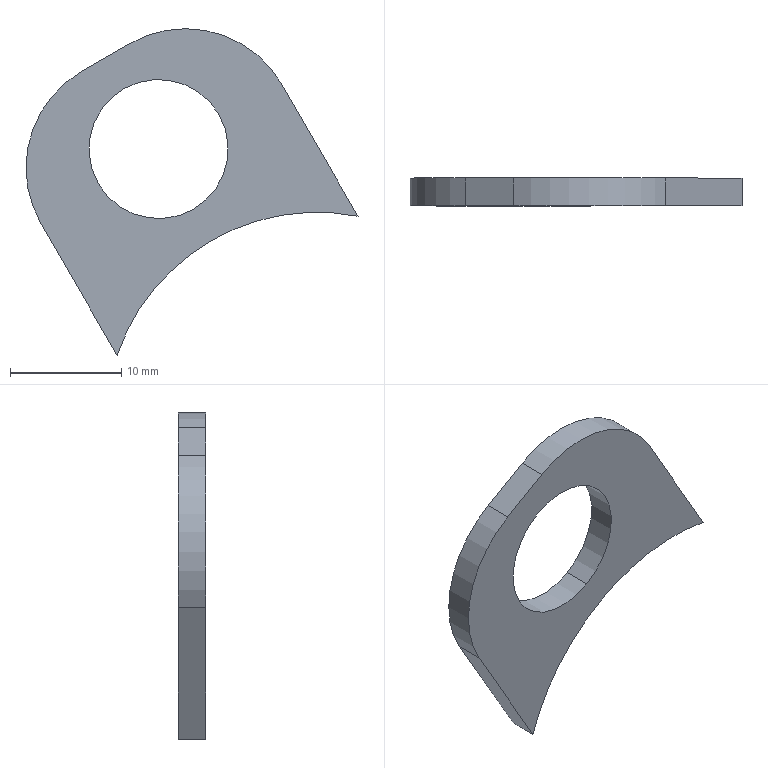Part | SolidWorks | features BaseBody 1 | 1 solid | 11 faces | box 29.836 x 2.5 x 29.357 mm | volume 865.731 mm3 | cylinder 6 | plane 5 | commonest cylinder face diameters 12.5 x2 20 x2 38 x2
STEP:
#1=CARTESIAN_POINT('',(212.375,172.7,29.663));
#2=VERTEX_POINT('',#1);
#3=CARTESIAN_POINT('',(218.625,172.7,18.837));
#4=VERTEX_POINT('',#3);
#5=CARTESIAN_POINT('',(215.5,172.7,24.25));
#6=DIRECTION('',(0.,-1.,0.));
#7=DIRECTION('',(0.5,0.,-0.866));
#8=AXIS2_PLACEMENT_3D('',#5,#6,#7);
#9=CIRCLE('',#8,6.25);
#10=EDGE_CURVE('',#2,#4,#9,.T.);
#11=ORIENTED_EDGE('',*,*,#10,.T.);
#12=CARTESIAN_POINT('',(218.625,175.2,18.837));
#13=VERTEX_POINT('',#12);
#14=CARTESIAN_POINT('',(218.625,172.7,18.837));
#15=DIRECTION('',(0.,1.,0.));
#16=VECTOR('',#15,1000.);
#17=LINE('',#14,#16);
#18=EDGE_CURVE('',#4,#13,#17,.T.);
#19=ORIENTED_EDGE('',*,*,#18,.T.);
#20=CARTESIAN_POINT('',(212.375,175.2,29.663));
#21=VERTEX_POINT('',#20);
#22=CARTESIAN_POINT('',(215.5,175.2,24.25));
#23=DIRECTION('',(0.,-1.,0.));
#24=DIRECTION('',(0.5,0.,-0.866));
#25=AXIS2_PLACEMENT_3D('',#22,#23,#24);
#26=CIRCLE('',#25,6.25);
#27=EDGE_CURVE('',#21,#13,#26,.T.);
#28=ORIENTED_EDGE('',*,*,#27,.F.);
#29=CARTESIAN_POINT('',(212.375,172.7,29.663));
#30=DIRECTION('',(0.,1.,0.));
#31=VECTOR('',#30,1000.);
#32=LINE('',#29,#31);
#33=EDGE_CURVE('',#2,#21,#32,.T.);
#34=ORIENTED_EDGE('',*,*,#33,.F.);
#35=EDGE_LOOP('',(#11,#19,#28,#34));
#36=FACE_OUTER_BOUND('',#35,.T.);
#37=CARTESIAN_POINT('',(215.5,172.7,24.25));
#38=DIRECTION('',(0.,1.,0.));
#39=DIRECTION('',(-0.5,0.,0.866));
#40=AXIS2_PLACEMENT_3D('',#37,#38,#39);
#41=CYLINDRICAL_SURFACE('',#40,6.25);
#42=ADVANCED_FACE('',(#36),#41,.F.);
#43=CARTESIAN_POINT('',(220.25,172.7,16.023));
#44=VERTEX_POINT('',#43);
#45=CARTESIAN_POINT('',(233.421,172.7,18.21));
#46=VERTEX_POINT('',#45);
#47=CARTESIAN_POINT('',(229.749,172.7,-0.4321));
#48=DIRECTION('',(0.,1.,0.));
#49=DIRECTION('',(0.5,0.,-0.866));
#50=AXIS2_PLACEMENT_3D('',#47,#48,#49);
#51=CIRCLE('',#50,19.);
#52=EDGE_CURVE('',#44,#46,#51,.T.);
#53=ORIENTED_EDGE('',*,*,#52,.F.);
#54=CARTESIAN_POINT('',(220.25,175.2,16.023));
#55=VERTEX_POINT('',#54);
#56=CARTESIAN_POINT('',(220.25,172.7,16.023));
#57=DIRECTION('',(0.,1.,0.));
#58=VECTOR('',#57,1000.);
#59=LINE('',#56,#58);
#60=EDGE_CURVE('',#44,#55,#59,.T.);
#61=ORIENTED_EDGE('',*,*,#60,.T.);
#62=CARTESIAN_POINT('',(233.421,175.2,18.21));
#63=VERTEX_POINT('',#62);
#64=CARTESIAN_POINT('',(229.749,175.2,-0.4321));
#65=DIRECTION('',(0.,1.,0.));
#66=DIRECTION('',(0.5,0.,-0.866));
#67=AXIS2_PLACEMENT_3D('',#64,#65,#66);
#68=CIRCLE('',#67,19.);
#69=EDGE_CURVE('',#55,#63,#68,.T.);
#70=ORIENTED_EDGE('',*,*,#69,.T.);
#71=CARTESIAN_POINT('',(233.421,172.7,18.21));
#72=DIRECTION('',(0.,1.,0.));
#73=VECTOR('',#72,1000.);
#74=LINE('',#71,#73);
#75=EDGE_CURVE('',#46,#63,#74,.T.);
#76=ORIENTED_EDGE('',*,*,#75,.F.);
#77=EDGE_LOOP('',(#53,#61,#70,#76));
#78=FACE_OUTER_BOUND('',#77,.T.);
#79=CARTESIAN_POINT('',(229.749,172.7,-0.4321));
#80=DIRECTION('',(0.,1.,0.));
#81=DIRECTION('',(-0.5,0.,0.866));
#82=AXIS2_PLACEMENT_3D('',#79,#80,#81);
#83=CYLINDRICAL_SURFACE('',#82,19.);
#84=ADVANCED_FACE('',(#78),#83,.F.);
#85=CARTESIAN_POINT('',(211.77,172.7,5.71));
#86=VERTEX_POINT('',#85);
#87=CARTESIAN_POINT('',(229.749,172.7,-0.4321));
#88=DIRECTION('',(0.,1.,0.));
#89=DIRECTION('',(0.5,0.,-0.866));
#90=AXIS2_PLACEMENT_3D('',#87,#88,#89);
#91=CIRCLE('',#90,19.);
#92=EDGE_CURVE('',#86,#44,#91,.T.);
#93=ORIENTED_EDGE('',*,*,#92,.T.);
#94=ORIENTED_EDGE('',*,*,#52,.T.);
#95=CARTESIAN_POINT('',(226.575,172.7,30.067));
#96=VERTEX_POINT('',#95);
#97=CARTESIAN_POINT('',(226.575,172.7,30.067));
#98=DIRECTION('',(-0.5,0.,0.866));
#99=VECTOR('',#98,1000.);
#100=LINE('',#97,#99);
#101=EDGE_CURVE('',#46,#96,#100,.T.);
#102=ORIENTED_EDGE('',*,*,#101,.T.);
#103=CARTESIAN_POINT('',(212.915,172.7,33.727));
#104=VERTEX_POINT('',#103);
#105=CARTESIAN_POINT('',(217.915,172.7,25.067));
#106=DIRECTION('',(0.,-1.,0.));
#107=DIRECTION('',(0.5,0.,-0.866));
#108=AXIS2_PLACEMENT_3D('',#105,#106,#107);
#109=CIRCLE('',#108,10.);
#110=EDGE_CURVE('',#96,#104,#109,.T.);
#111=ORIENTED_EDGE('',*,*,#110,.T.);
#112=CARTESIAN_POINT('',(208.585,172.7,31.227));
#113=VERTEX_POINT('',#112);
#114=CARTESIAN_POINT('',(212.915,172.7,33.727));
#115=DIRECTION('',(-0.866,0.,-0.5));
#116=VECTOR('',#115,1000.);
#117=LINE('',#114,#116);
#118=EDGE_CURVE('',#104,#113,#117,.T.);
#119=ORIENTED_EDGE('',*,*,#118,.T.);
#120=CARTESIAN_POINT('',(204.925,172.7,17.567));
#121=VERTEX_POINT('',#120);
#122=CARTESIAN_POINT('',(213.585,172.7,22.567));
#123=DIRECTION('',(0.,-1.,0.));
#124=DIRECTION('',(-0.5,0.,0.866));
#125=AXIS2_PLACEMENT_3D('',#122,#123,#124);
#126=CIRCLE('',#125,10.);
#127=EDGE_CURVE('',#113,#121,#126,.T.);
#128=ORIENTED_EDGE('',*,*,#127,.T.);
#129=CARTESIAN_POINT('',(204.925,172.7,17.567));
#130=DIRECTION('',(0.5,0.,-0.866));
#131=VECTOR('',#130,1000.);
#132=LINE('',#129,#131);
#133=EDGE_CURVE('',#121,#86,#132,.T.);
#134=ORIENTED_EDGE('',*,*,#133,.T.);
#135=EDGE_LOOP('',(#93,#94,#102,#111,#119,#128,#134));
#136=FACE_OUTER_BOUND('',#135,.T.);
#137=ORIENTED_EDGE('',*,*,#10,.F.);
#138=CARTESIAN_POINT('',(215.5,172.7,24.25));
#139=DIRECTION('',(0.,-1.,0.));
#140=DIRECTION('',(0.5,0.,-0.866));
#141=AXIS2_PLACEMENT_3D('',#138,#139,#140);
#142=CIRCLE('',#141,6.25);
#143=EDGE_CURVE('',#4,#2,#142,.T.);
#144=ORIENTED_EDGE('',*,*,#143,.F.);
#145=EDGE_LOOP('',(#137,#144));
#146=FACE_BOUND('',#145,.T.);
#147=CARTESIAN_POINT('',(229.749,172.7,-0.4321));
#148=DIRECTION('',(0.,-1.,0.));
#149=DIRECTION('',(0.5,0.,-0.866));
#150=AXIS2_PLACEMENT_3D('',#147,#148,#149);
#151=PLANE('',#150);
#152=ADVANCED_FACE('',(#136,#146),#151,.T.);
#153=CARTESIAN_POINT('',(211.77,175.2,5.71));
#154=VERTEX_POINT('',#153);
#155=CARTESIAN_POINT('',(229.749,175.2,-0.4321));
#156=DIRECTION('',(0.,1.,0.));
#157=DIRECTION('',(0.5,0.,-0.866));
#158=AXIS2_PLACEMENT_3D('',#155,#156,#157);
#159=CIRCLE('',#158,19.);
#160=EDGE_CURVE('',#154,#55,#159,.T.);
#161=ORIENTED_EDGE('',*,*,#160,.F.);
#162=CARTESIAN_POINT('',(204.925,175.2,17.567));
#163=VERTEX_POINT('',#162);
#164=CARTESIAN_POINT('',(204.925,175.2,17.567));
#165=DIRECTION('',(0.5,0.,-0.866));
#166=VECTOR('',#165,1000.);
#167=LINE('',#164,#166);
#168=EDGE_CURVE('',#163,#154,#167,.T.);
#169=ORIENTED_EDGE('',*,*,#168,.F.);
#170=CARTESIAN_POINT('',(208.585,175.2,31.227));
#171=VERTEX_POINT('',#170);
#172=CARTESIAN_POINT('',(213.585,175.2,22.567));
#173=DIRECTION('',(0.,-1.,0.));
#174=DIRECTION('',(-0.5,0.,0.866));
#175=AXIS2_PLACEMENT_3D('',#172,#173,#174);
#176=CIRCLE('',#175,10.);
#177=EDGE_CURVE('',#171,#163,#176,.T.);
#178=ORIENTED_EDGE('',*,*,#177,.F.);
#179=CARTESIAN_POINT('',(212.915,175.2,33.727));
#180=VERTEX_POINT('',#179);
#181=CARTESIAN_POINT('',(212.915,175.2,33.727));
#182=DIRECTION('',(-0.866,0.,-0.5));
#183=VECTOR('',#182,1000.);
#184=LINE('',#181,#183);
#185=EDGE_CURVE('',#180,#171,#184,.T.);
#186=ORIENTED_EDGE('',*,*,#185,.F.);
#187=CARTESIAN_POINT('',(226.575,175.2,30.067));
#188=VERTEX_POINT('',#187);
#189=CARTESIAN_POINT('',(217.915,175.2,25.067));
#190=DIRECTION('',(0.,-1.,0.));
#191=DIRECTION('',(0.5,0.,-0.866));
#192=AXIS2_PLACEMENT_3D('',#189,#190,#191);
#193=CIRCLE('',#192,10.);
#194=EDGE_CURVE('',#188,#180,#193,.T.);
#195=ORIENTED_EDGE('',*,*,#194,.F.);
#196=CARTESIAN_POINT('',(226.575,175.2,30.067));
#197=DIRECTION('',(-0.5,0.,0.866));
#198=VECTOR('',#197,1000.);
#199=LINE('',#196,#198);
#200=EDGE_CURVE('',#63,#188,#199,.T.);
#201=ORIENTED_EDGE('',*,*,#200,.F.);
#202=ORIENTED_EDGE('',*,*,#69,.F.);
#203=EDGE_LOOP('',(#161,#169,#178,#186,#195,#201,#202));
#204=FACE_OUTER_BOUND('',#203,.T.);
#205=ORIENTED_EDGE('',*,*,#27,.T.);
#206=CARTESIAN_POINT('',(215.5,175.2,24.25));
#207=DIRECTION('',(0.,-1.,0.));
#208=DIRECTION('',(0.5,0.,-0.866));
#209=AXIS2_PLACEMENT_3D('',#206,#207,#208);
#210=CIRCLE('',#209,6.25);
#211=EDGE_CURVE('',#13,#21,#210,.T.);
#212=ORIENTED_EDGE('',*,*,#211,.T.);
#213=EDGE_LOOP('',(#205,#212));
#214=FACE_BOUND('',#213,.T.);
#215=CARTESIAN_POINT('',(229.749,175.2,-0.4321));
#216=DIRECTION('',(0.,-1.,0.));
#217=DIRECTION('',(0.5,0.,-0.866));
#218=AXIS2_PLACEMENT_3D('',#215,#216,#217);
#219=PLANE('',#218);
#220=ADVANCED_FACE('',(#204,#214),#219,.F.);
#221=ORIENTED_EDGE('',*,*,#60,.F.);
#222=ORIENTED_EDGE('',*,*,#92,.F.);
#223=CARTESIAN_POINT('',(211.77,172.7,5.71));
#224=DIRECTION('',(0.,1.,0.));
#225=VECTOR('',#224,1000.);
#226=LINE('',#223,#225);
#227=EDGE_CURVE('',#86,#154,#226,.T.);
#228=ORIENTED_EDGE('',*,*,#227,.T.);
#229=ORIENTED_EDGE('',*,*,#160,.T.);
#230=EDGE_LOOP('',(#221,#222,#228,#229));
#231=FACE_OUTER_BOUND('',#230,.T.);
#232=CARTESIAN_POINT('',(229.749,172.7,-0.4321));
#233=DIRECTION('',(0.,1.,0.));
#234=DIRECTION('',(-0.5,0.,0.866));
#235=AXIS2_PLACEMENT_3D('',#232,#233,#234);
#236=CYLINDRICAL_SURFACE('',#235,19.);
#237=ADVANCED_FACE('',(#231),#236,.F.);
#238=ORIENTED_EDGE('',*,*,#200,.T.);
#239=CARTESIAN_POINT('',(226.575,172.7,30.067));
#240=DIRECTION('',(0.,1.,0.));
#241=VECTOR('',#240,1000.);
#242=LINE('',#239,#241);
#243=EDGE_CURVE('',#96,#188,#242,.T.);
#244=ORIENTED_EDGE('',*,*,#243,.F.);
#245=ORIENTED_EDGE('',*,*,#101,.F.);
#246=ORIENTED_EDGE('',*,*,#75,.T.);
#247=EDGE_LOOP('',(#238,#244,#245,#246));
#248=FACE_OUTER_BOUND('',#247,.T.);
#249=CARTESIAN_POINT('',(226.575,172.7,30.067));
#250=DIRECTION('',(-0.866,0.,-0.5));
#251=DIRECTION('',(0.5,0.,-0.866));
#252=AXIS2_PLACEMENT_3D('',#249,#250,#251);
#253=PLANE('',#252);
#254=ADVANCED_FACE('',(#248),#253,.F.);
#255=ORIENTED_EDGE('',*,*,#194,.T.);
#256=CARTESIAN_POINT('',(212.915,172.7,33.727));
#257=DIRECTION('',(0.,1.,0.));
#258=VECTOR('',#257,1000.);
#259=LINE('',#256,#258);
#260=EDGE_CURVE('',#104,#180,#259,.T.);
#261=ORIENTED_EDGE('',*,*,#260,.F.);
#262=ORIENTED_EDGE('',*,*,#110,.F.);
#263=ORIENTED_EDGE('',*,*,#243,.T.);
#264=EDGE_LOOP('',(#255,#261,#262,#263));
#265=FACE_OUTER_BOUND('',#264,.T.);
#266=CARTESIAN_POINT('',(217.915,172.7,25.067));
#267=DIRECTION('',(0.,1.,0.));
#268=DIRECTION('',(-0.5,0.,0.866));
#269=AXIS2_PLACEMENT_3D('',#266,#267,#268);
#270=CYLINDRICAL_SURFACE('',#269,10.);
#271=ADVANCED_FACE('',(#265),#270,.T.);
#272=ORIENTED_EDGE('',*,*,#185,.T.);
#273=CARTESIAN_POINT('',(208.585,172.7,31.227));
#274=DIRECTION('',(0.,1.,0.));
#275=VECTOR('',#274,1000.);
#276=LINE('',#273,#275);
#277=EDGE_CURVE('',#113,#171,#276,.T.);
#278=ORIENTED_EDGE('',*,*,#277,.F.);
#279=ORIENTED_EDGE('',*,*,#118,.F.);
#280=ORIENTED_EDGE('',*,*,#260,.T.);
#281=EDGE_LOOP('',(#272,#278,#279,#280));
#282=FACE_OUTER_BOUND('',#281,.T.);
#283=CARTESIAN_POINT('',(212.915,172.7,33.727));
#284=DIRECTION('',(0.5,0.,-0.866));
#285=DIRECTION('',(0.,1.,0.));
#286=AXIS2_PLACEMENT_3D('',#283,#284,#285);
#287=PLANE('',#286);
#288=ADVANCED_FACE('',(#282),#287,.F.);
#289=ORIENTED_EDGE('',*,*,#177,.T.);
#290=CARTESIAN_POINT('',(204.925,172.7,17.567));
#291=DIRECTION('',(0.,1.,0.));
#292=VECTOR('',#291,1000.);
#293=LINE('',#290,#292);
#294=EDGE_CURVE('',#121,#163,#293,.T.);
#295=ORIENTED_EDGE('',*,*,#294,.F.);
#296=ORIENTED_EDGE('',*,*,#127,.F.);
#297=ORIENTED_EDGE('',*,*,#277,.T.);
#298=EDGE_LOOP('',(#289,#295,#296,#297));
#299=FACE_OUTER_BOUND('',#298,.T.);
#300=CARTESIAN_POINT('',(213.585,172.7,22.567));
#301=DIRECTION('',(0.,1.,0.));
#302=DIRECTION('',(-0.5,0.,0.866));
#303=AXIS2_PLACEMENT_3D('',#300,#301,#302);
#304=CYLINDRICAL_SURFACE('',#303,10.);
#305=ADVANCED_FACE('',(#299),#304,.T.);
#306=ORIENTED_EDGE('',*,*,#168,.T.);
#307=ORIENTED_EDGE('',*,*,#227,.F.);
#308=ORIENTED_EDGE('',*,*,#133,.F.);
#309=ORIENTED_EDGE('',*,*,#294,.T.);
#310=EDGE_LOOP('',(#306,#307,#308,#309));
#311=FACE_OUTER_BOUND('',#310,.T.);
#312=CARTESIAN_POINT('',(204.925,172.7,17.567));
#313=DIRECTION('',(0.866,0.,0.5));
#314=DIRECTION('',(-0.5,0.,0.866));
#315=AXIS2_PLACEMENT_3D('',#312,#313,#314);
#316=PLANE('',#315);
#317=ADVANCED_FACE('',(#311),#316,.F.);
#318=ORIENTED_EDGE('',*,*,#18,.F.);
#319=ORIENTED_EDGE('',*,*,#143,.T.);
#320=ORIENTED_EDGE('',*,*,#33,.T.);
#321=ORIENTED_EDGE('',*,*,#211,.F.);
#322=EDGE_LOOP('',(#318,#319,#320,#321));
#323=FACE_OUTER_BOUND('',#322,.T.);
#324=CARTESIAN_POINT('',(215.5,172.7,24.25));
#325=DIRECTION('',(0.,1.,0.));
#326=DIRECTION('',(-0.5,0.,0.866));
#327=AXIS2_PLACEMENT_3D('',#324,#325,#326);
#328=CYLINDRICAL_SURFACE('',#327,6.25);
#329=ADVANCED_FACE('',(#323),#328,.F.);
#330=CLOSED_SHELL('',(#42,#84,#152,#220,#237,#254,#271,#288,#305,#317,#329));
#331=MANIFOLD_SOLID_BREP('',#330);
#332=CARTESIAN_POINT('',(0.,0.,0.));
#333=DIRECTION('',(0.,0.,1.));
#334=DIRECTION('',(1.,0.,0.));
#335=AXIS2_PLACEMENT_3D('',#332,#333,#334);
#336=(LENGTH_UNIT()NAMED_UNIT(*)SI_UNIT(.MILLI.,.METRE.));
#337=UNCERTAINTY_MEASURE_WITH_UNIT(LENGTH_MEASURE(0.00001),#336,'','');
#338=(NAMED_UNIT(*)PLANE_ANGLE_UNIT()SI_UNIT($,.RADIAN.));
#339=(NAMED_UNIT(*)SI_UNIT($,.STERADIAN.)SOLID_ANGLE_UNIT());
#340=(GEOMETRIC_REPRESENTATION_CONTEXT(3)GLOBAL_UNCERTAINTY_ASSIGNED_CONTEXT((#337))GLOBAL_UNIT_ASSIGNED_CONTEXT((#336,#338,#339))REPRESENTATION_CONTEXT('',''));
#341=ADVANCED_BREP_SHAPE_REPRESENTATION('',(#331,#335),#340);